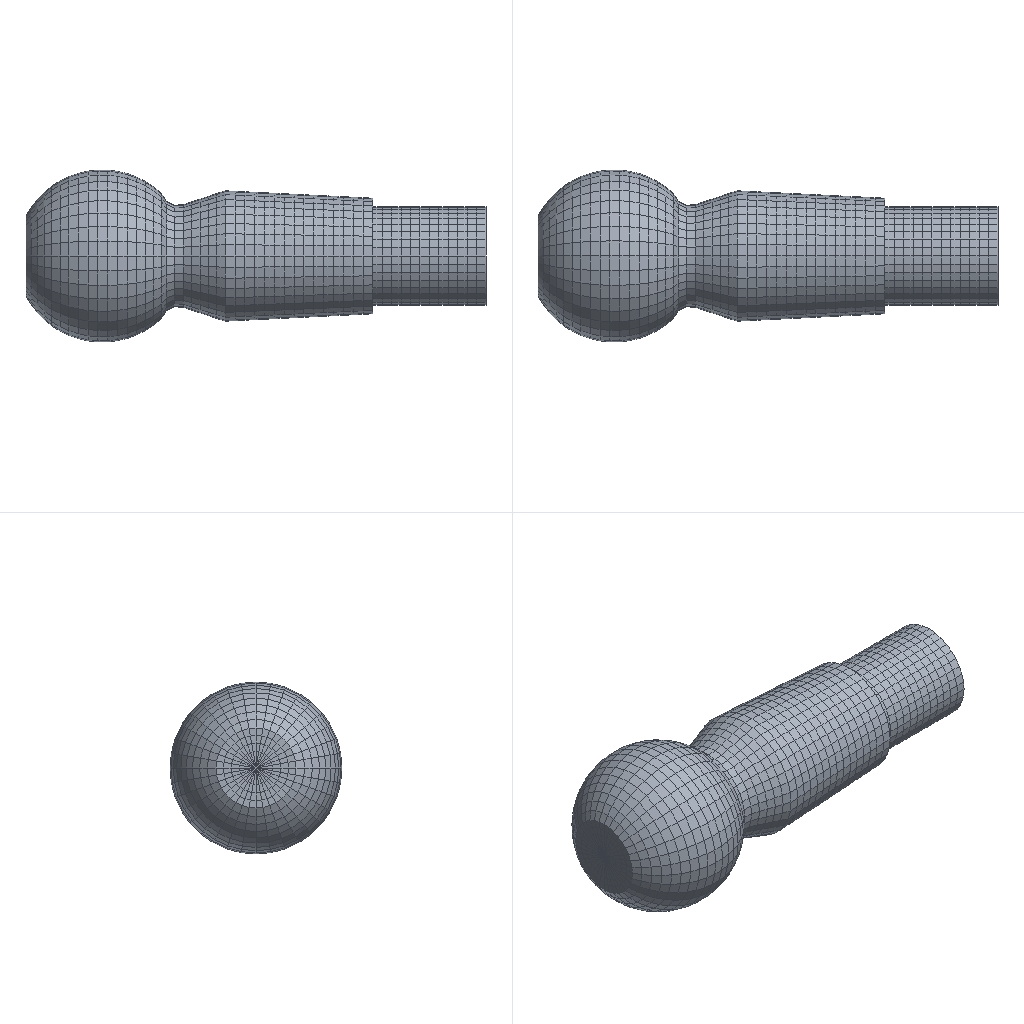Simulation study | abaqus
Set-up summary:
category,name,step,type,value,unit,region
solver,abaqus,,Abaqus/CAE 2024
units,mm-N-s-tonne (MPa),,inferred,E=210000 density=
analysis,Step-1,,static,nlgeom=True; time_period=1
mesh,nodes,,,12325
mesh,elements,,,12096
element_type,C3D8R,,,10224
element_type,C3D6,,,1872
material,Steel_40Cr,,E,210000
material,Steel_40Cr,,nu,0.3
material,Steel_40Cr,,yield,918
material,Steel_40Cr,,behaviors,plastic
section,Steel_40Cr,,solid section,,,Set-13
load,Load-1,Step-1,concentrated force,"100 [dir=(0, 1, 0)]",,Set-3
bc,BC-1,initial,fixed,"[dofs=ry,rz,x,y,z n=5]",,Set-2
constraint,coupling,,,1
Abaqus input file, long lists of numbers shortened:
*Heading
** Job name: deck Model name: qiuxiao
** Generated by: Abaqus/CAE 2024
*Preprint, echo=NO, model=NO, history=NO, contact=NO
**
** PARTS
**
*Part, name=qiuxiao
*Node
      1,        -15.5,           0.,           0.
      2,          29.,           0.,           0.
** (12322 more lines like these left out)
*Element, type=C3D8R
   1,   38,  573,  594,   37,  958, 3557, 3578,  959
   2,  573,  574,  595,  594, 3557, 3558, 3579, 3578
** (10222 more lines like these left out)
*Element, type=C3D6
1513,   88,  615, 3599,    2,   36,  960
1514,   87,  616, 3600,   88,  615, 3599
** (1870 more lines like these left out)
*Nset, nset=Set-13, generate
     1,  12324,      1
*Elset, elset=Set-13, generate
     1,  12096,      1
** Section: qiuxiao
*Solid Section, elset=Set-13, material=Steel_40Cr
,
*End Part
**
**
** ASSEMBLY
**
*Assembly, name=Assembly
**
*Instance, name=qiuxiao-1, part=qiuxiao
*End Instance
**
*Node
      1,           0.,           0.,           0.
*Nset, nset=Set-2, instance=qiuxiao-1
    3,    8,   13,   18,   23,   27,   32,   35,   97,   98,   99,  100,  101,  102,  103,  104
  169,  170,  171,  172,  173,  174,  175,  176,  241,  242,  243,  244,  245,  246,  247,  248
** (30 more lines like these left out)
*Elset, elset=Set-2, instance=qiuxiao-1
  7001,  7004,  7011,  7015,  7017,  7023,  7037,  7058,  7061,  7063,  7064,  7065,  7068,  7117,  7120,  7127
  7131,  7133,  7139,  7153,  7174,  7177,  7179,  7180,  7181,  7184,  7233,  7236,  7243,  7247,  7249,  7255
** (28 more lines like these left out)
*Nset, nset=Set-3
 1,
*Nset, nset=m_Set-1
 1,
*Elset, elset=_s_Surf-1_S6, internal, instance=qiuxiao-1
   55,   57,  110,  223,  225,  278,  391,  393,  446,  559,  561,  614,  727,  729,  782,  895
  897,  950, 1063, 1065, 1118, 1231, 1233, 1286, 1399, 1401, 1454, 1801, 1803, 1856, 1969, 1971
** (5 more lines like these left out)
*Elset, elset=_s_Surf-1_S4, internal, instance=qiuxiao-1
   68,   84,   85,   86,   87,   96,   98,  100,  102,  105,  107,  109,  236,  252,  253,  254
  255,  264,  266,  268,  270,  273,  275,  277,  404,  420,  421,  422,  423,  432,  434,  436
** (25 more lines like these left out)
*Elset, elset=_s_Surf-1_S3, internal, instance=qiuxiao-1
   76,  244,  412,  580,  748,  916, 1084, 1252, 1420, 1822, 1990, 2158, 2326, 2494, 2662, 2830
 2998, 3166, 3568, 3736, 3904, 4072, 4240, 4408, 4576, 4744, 4912, 5314, 5482, 5650, 5818, 5986
** (1 more lines like these left out)
*Surface, type=ELEMENT, name=s_Surf-1
_s_Surf-1_S6, S6
_s_Surf-1_S4, S4
_s_Surf-1_S3, S3
** Constraint: Constraint-1
*Coupling, constraint name=Constraint-1, ref node=m_Set-1, surface=s_Surf-1
*Distributing, weighting method=UNIFORM
*End Assembly
**
** MATERIALS
**
*Material, name=Steel_40Cr
*Elastic
210000., 0.3
*Plastic
918.,0.
**
** BOUNDARY CONDITIONS
**
** Name: BC-1 Type: Displacement/Rotation
*Boundary
Set-2, 1, 1
Set-2, 2, 2
Set-2, 3, 3
Set-2, 5, 5
Set-2, 6, 6
** ----------------------------------------------------------------
**
** STEP: Step-1
**
*Step, name=Step-1, nlgeom=YES
*Static, riks
1., 1., 1e-05, , ,
**
** LOADS
**
** Name: Load-1   Type: Concentrated force
*Cload
Set-3, 2, 100.
**
** OUTPUT REQUESTS
**
*Restart, write, frequency=0
**
** FIELD OUTPUT: F-Output-1
**
*Output, field, variable=PRESELECT
**
** HISTORY OUTPUT: H-Output-1
**
*Output, history, variable=PRESELECT
*End Step
Results summary:
result,odb.job_status,,,JOB_STATUS_COMPLETED_SUCCESSFULLY,"consistent, unstated (Abaqus has no unit system)"
result,steps[0].procedure,Step-1,,"*STATIC, RIKS","consistent, unstated (Abaqus has no unit system)"
result,steps[0].time_period,Step-1,,183833,"consistent, unstated (Abaqus has no unit system)"
result,steps[0].n_frames,Step-1,,101,"consistent, unstated (Abaqus has no unit system)"
result,steps[0].last_frame.id,Step-1,,100,"consistent, unstated (Abaqus has no unit system)"
result,steps[0].last_frame.value,Step-1,,183833,"consistent, unstated (Abaqus has no unit system)"
result,steps[0].last_frame.description,Step-1,,Increment    100: Arc Length =   1.8383E+05,"consistent, unstated (Abaqus has no unit system)"
result,steps[0].max_U_magnitude,Step-1,,84.879,"consistent, unstated (Abaqus has no unit system)"
result,steps[0].max_S_mises,Step-1,,918.001,"consistent, unstated (Abaqus has no unit system)"
result,steps[0].RF_sum[1],Step-1,,0.1557,"consistent, unstated (Abaqus has no unit system)"
result,steps[0].RF_sum[2],Step-1,,-198952,"consistent, unstated (Abaqus has no unit system)"
result,steps[0].RF_sum[3],Step-1,,-0.002977,"consistent, unstated (Abaqus has no unit system)"